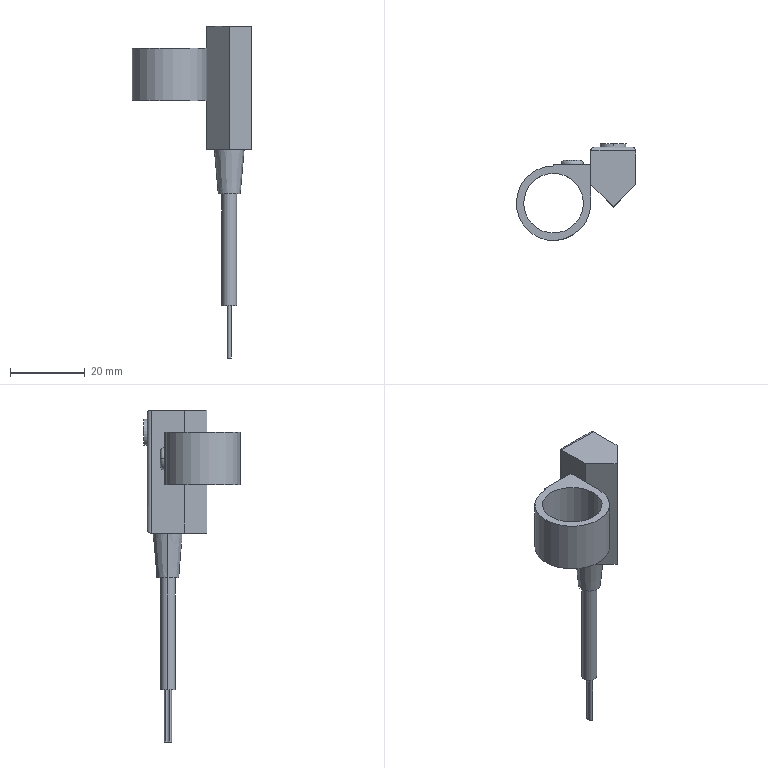Part | STEP file | CDS1FN160-250-A54Z_A5_A6_F5_J5_ForLargeBore | 1 solid | 43 faces | box 32 x 26 x 89 mm | volume 7994 mm3 | plane 22 | cylinder 17 | torus 2 | cone 2 | commonest cylinder face diameters 1 x4 2 x4 3 x2 4 x2 7 x2 16 x2